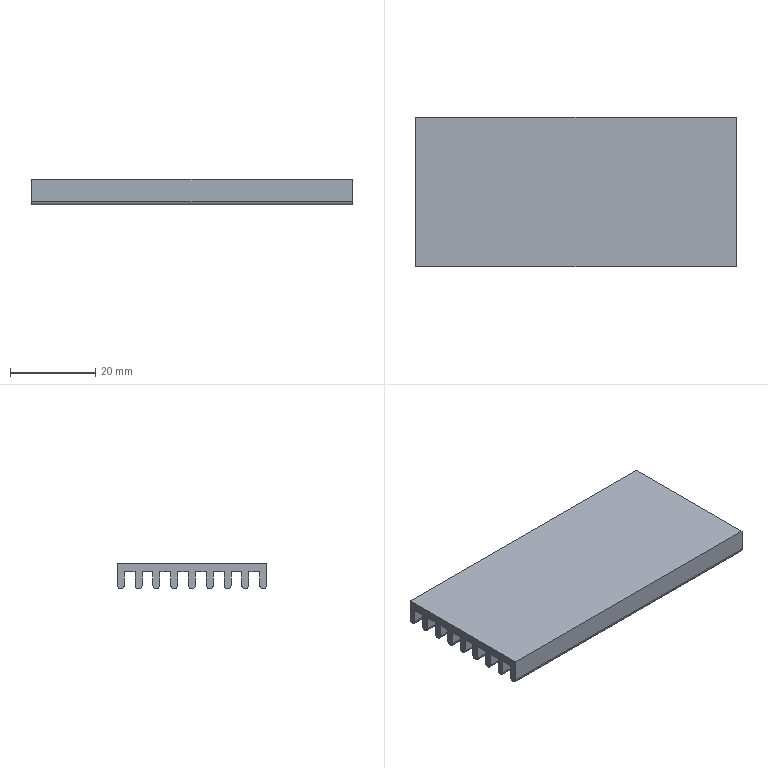Part | SolidWorks | features Fillet 9, Cut 1, Extrusion 1, LPattern 1 | 1 solid | 38 faces | box 75 x 35 x 6 mm | volume 9439 mm3 | plane 29 | cylinder 9 | commonest cylinder face diameters 1.62 x8 1.64 x1
STEP:
#1=CARTESIAN_POINT('',(37.5,-15.86,0.82));
#2=VERTEX_POINT('',#1);
#3=CARTESIAN_POINT('',(-37.5,-15.86,0.82));
#4=VERTEX_POINT('',#3);
#5=CARTESIAN_POINT('',(37.5,-15.86,0.82));
#6=DIRECTION('',(-1.,0.,0.));
#7=VECTOR('',#6,1000.);
#8=LINE('',#5,#7);
#9=EDGE_CURVE('',#2,#4,#8,.T.);
#10=ORIENTED_EDGE('',*,*,#9,.F.);
#11=CARTESIAN_POINT('',(37.5,-17.5,0.82));
#12=VERTEX_POINT('',#11);
#13=CARTESIAN_POINT('',(37.5,-16.68,0.82));
#14=DIRECTION('',(1.,0.,0.));
#15=DIRECTION('',(0.,-1.,0.));
#16=AXIS2_PLACEMENT_3D('',#13,#14,#15);
#17=CIRCLE('',#16,0.82);
#18=EDGE_CURVE('',#12,#2,#17,.T.);
#19=ORIENTED_EDGE('',*,*,#18,.F.);
#20=CARTESIAN_POINT('',(-37.5,-17.5,0.82));
#21=VERTEX_POINT('',#20);
#22=CARTESIAN_POINT('',(-37.5,-17.5,0.82));
#23=DIRECTION('',(1.,0.,0.));
#24=VECTOR('',#23,1000.);
#25=LINE('',#22,#24);
#26=EDGE_CURVE('',#21,#12,#25,.T.);
#27=ORIENTED_EDGE('',*,*,#26,.F.);
#28=CARTESIAN_POINT('',(-37.5,-16.68,0.82));
#29=DIRECTION('',(-1.,0.,0.));
#30=DIRECTION('',(0.,1.,0.));
#31=AXIS2_PLACEMENT_3D('',#28,#29,#30);
#32=CIRCLE('',#31,0.82);
#33=EDGE_CURVE('',#4,#21,#32,.T.);
#34=ORIENTED_EDGE('',*,*,#33,.F.);
#35=EDGE_LOOP('',(#10,#19,#27,#34));
#36=FACE_OUTER_BOUND('',#35,.T.);
#37=CARTESIAN_POINT('',(37.5,-16.68,0.82));
#38=DIRECTION('',(-1.,0.,0.));
#39=DIRECTION('',(0.,0.,1.));
#40=AXIS2_PLACEMENT_3D('',#37,#38,#39);
#41=CYLINDRICAL_SURFACE('',#40,0.82);
#42=ADVANCED_FACE('',(#36),#41,.T.);
#43=CARTESIAN_POINT('',(37.5,-11.69,0.81));
#44=VERTEX_POINT('',#43);
#45=CARTESIAN_POINT('',(-37.5,-11.69,0.81));
#46=VERTEX_POINT('',#45);
#47=CARTESIAN_POINT('',(37.5,-11.69,0.81));
#48=DIRECTION('',(-1.,0.,0.));
#49=VECTOR('',#48,1000.);
#50=LINE('',#47,#49);
#51=EDGE_CURVE('',#44,#46,#50,.T.);
#52=ORIENTED_EDGE('',*,*,#51,.F.);
#53=CARTESIAN_POINT('',(37.5,-13.31,0.81));
#54=VERTEX_POINT('',#53);
#55=CARTESIAN_POINT('',(37.5,-12.5,0.81));
#56=DIRECTION('',(1.,0.,0.));
#57=DIRECTION('',(0.,-1.,0.));
#58=AXIS2_PLACEMENT_3D('',#55,#56,#57);
#59=CIRCLE('',#58,0.81);
#60=EDGE_CURVE('',#54,#44,#59,.T.);
#61=ORIENTED_EDGE('',*,*,#60,.F.);
#62=CARTESIAN_POINT('',(-37.5,-13.31,0.81));
#63=VERTEX_POINT('',#62);
#64=CARTESIAN_POINT('',(37.5,-13.31,0.81));
#65=DIRECTION('',(1.,0.,0.));
#66=VECTOR('',#65,1000.);
#67=LINE('',#64,#66);
#68=EDGE_CURVE('',#63,#54,#67,.T.);
#69=ORIENTED_EDGE('',*,*,#68,.F.);
#70=CARTESIAN_POINT('',(-37.5,-12.5,0.81));
#71=DIRECTION('',(-1.,0.,0.));
#72=DIRECTION('',(0.,1.,0.));
#73=AXIS2_PLACEMENT_3D('',#70,#71,#72);
#74=CIRCLE('',#73,0.81);
#75=EDGE_CURVE('',#46,#63,#74,.T.);
#76=ORIENTED_EDGE('',*,*,#75,.F.);
#77=EDGE_LOOP('',(#52,#61,#69,#76));
#78=FACE_OUTER_BOUND('',#77,.T.);
#79=CARTESIAN_POINT('',(37.5,-12.5,0.81));
#80=DIRECTION('',(-1.,0.,0.));
#81=DIRECTION('',(0.,0.,1.));
#82=AXIS2_PLACEMENT_3D('',#79,#80,#81);
#83=CYLINDRICAL_SURFACE('',#82,0.81);
#84=ADVANCED_FACE('',(#78),#83,.T.);
#85=CARTESIAN_POINT('',(37.5,-7.52,0.81));
#86=VERTEX_POINT('',#85);
#87=CARTESIAN_POINT('',(-37.5,-7.52,0.81));
#88=VERTEX_POINT('',#87);
#89=CARTESIAN_POINT('',(37.5,-7.52,0.81));
#90=DIRECTION('',(-1.,0.,0.));
#91=VECTOR('',#90,1000.);
#92=LINE('',#89,#91);
#93=EDGE_CURVE('',#86,#88,#92,.T.);
#94=ORIENTED_EDGE('',*,*,#93,.F.);
#95=CARTESIAN_POINT('',(37.5,-9.14,0.81));
#96=VERTEX_POINT('',#95);
#97=CARTESIAN_POINT('',(37.5,-8.33,0.81));
#98=DIRECTION('',(1.,0.,0.));
#99=DIRECTION('',(0.,-1.,0.));
#100=AXIS2_PLACEMENT_3D('',#97,#98,#99);
#101=CIRCLE('',#100,0.81);
#102=EDGE_CURVE('',#96,#86,#101,.T.);
#103=ORIENTED_EDGE('',*,*,#102,.F.);
#104=CARTESIAN_POINT('',(-37.5,-9.14,0.81));
#105=VERTEX_POINT('',#104);
#106=CARTESIAN_POINT('',(37.5,-9.14,0.81));
#107=DIRECTION('',(1.,0.,0.));
#108=VECTOR('',#107,1000.);
#109=LINE('',#106,#108);
#110=EDGE_CURVE('',#105,#96,#109,.T.);
#111=ORIENTED_EDGE('',*,*,#110,.F.);
#112=CARTESIAN_POINT('',(-37.5,-8.33,0.81));
#113=DIRECTION('',(-1.,0.,0.));
#114=DIRECTION('',(0.,1.,0.));
#115=AXIS2_PLACEMENT_3D('',#112,#113,#114);
#116=CIRCLE('',#115,0.81);
#117=EDGE_CURVE('',#88,#105,#116,.T.);
#118=ORIENTED_EDGE('',*,*,#117,.F.);
#119=EDGE_LOOP('',(#94,#103,#111,#118));
#120=FACE_OUTER_BOUND('',#119,.T.);
#121=CARTESIAN_POINT('',(37.5,-8.33,0.81));
#122=DIRECTION('',(-1.,0.,0.));
#123=DIRECTION('',(0.,0.,1.));
#124=AXIS2_PLACEMENT_3D('',#121,#122,#123);
#125=CYLINDRICAL_SURFACE('',#124,0.81);
#126=ADVANCED_FACE('',(#120),#125,.T.);
#127=CARTESIAN_POINT('',(37.5,-3.35,0.81));
#128=VERTEX_POINT('',#127);
#129=CARTESIAN_POINT('',(-37.5,-3.35,0.81));
#130=VERTEX_POINT('',#129);
#131=CARTESIAN_POINT('',(37.5,-3.35,0.81));
#132=DIRECTION('',(-1.,0.,0.));
#133=VECTOR('',#132,1000.);
#134=LINE('',#131,#133);
#135=EDGE_CURVE('',#128,#130,#134,.T.);
#136=ORIENTED_EDGE('',*,*,#135,.F.);
#137=CARTESIAN_POINT('',(37.5,-4.97,0.81));
#138=VERTEX_POINT('',#137);
#139=CARTESIAN_POINT('',(37.5,-4.16,0.81));
#140=DIRECTION('',(1.,0.,0.));
#141=DIRECTION('',(0.,-1.,0.));
#142=AXIS2_PLACEMENT_3D('',#139,#140,#141);
#143=CIRCLE('',#142,0.81);
#144=EDGE_CURVE('',#138,#128,#143,.T.);
#145=ORIENTED_EDGE('',*,*,#144,.F.);
#146=CARTESIAN_POINT('',(-37.5,-4.97,0.81));
#147=VERTEX_POINT('',#146);
#148=CARTESIAN_POINT('',(37.5,-4.97,0.81));
#149=DIRECTION('',(1.,0.,0.));
#150=VECTOR('',#149,1000.);
#151=LINE('',#148,#150);
#152=EDGE_CURVE('',#147,#138,#151,.T.);
#153=ORIENTED_EDGE('',*,*,#152,.F.);
#154=CARTESIAN_POINT('',(-37.5,-4.16,0.81));
#155=DIRECTION('',(-1.,0.,0.));
#156=DIRECTION('',(0.,1.,0.));
#157=AXIS2_PLACEMENT_3D('',#154,#155,#156);
#158=CIRCLE('',#157,0.81);
#159=EDGE_CURVE('',#130,#147,#158,.T.);
#160=ORIENTED_EDGE('',*,*,#159,.F.);
#161=EDGE_LOOP('',(#136,#145,#153,#160));
#162=FACE_OUTER_BOUND('',#161,.T.);
#163=CARTESIAN_POINT('',(37.5,-4.16,0.81));
#164=DIRECTION('',(-1.,0.,0.));
#165=DIRECTION('',(0.,0.,1.));
#166=AXIS2_PLACEMENT_3D('',#163,#164,#165);
#167=CYLINDRICAL_SURFACE('',#166,0.81);
#168=ADVANCED_FACE('',(#162),#167,.T.);
#169=CARTESIAN_POINT('',(37.5,0.82,0.81));
#170=VERTEX_POINT('',#169);
#171=CARTESIAN_POINT('',(-37.5,0.82,0.81));
#172=VERTEX_POINT('',#171);
#173=CARTESIAN_POINT('',(37.5,0.82,0.81));
#174=DIRECTION('',(-1.,0.,0.));
#175=VECTOR('',#174,1000.);
#176=LINE('',#173,#175);
#177=EDGE_CURVE('',#170,#172,#176,.T.);
#178=ORIENTED_EDGE('',*,*,#177,.F.);
#179=CARTESIAN_POINT('',(37.5,-0.8,0.81));
#180=VERTEX_POINT('',#179);
#181=CARTESIAN_POINT('',(37.5,0.01,0.81));
#182=DIRECTION('',(1.,0.,0.));
#183=DIRECTION('',(0.,-1.,0.));
#184=AXIS2_PLACEMENT_3D('',#181,#182,#183);
#185=CIRCLE('',#184,0.81);
#186=EDGE_CURVE('',#180,#170,#185,.T.);
#187=ORIENTED_EDGE('',*,*,#186,.F.);
#188=CARTESIAN_POINT('',(-37.5,-0.8,0.81));
#189=VERTEX_POINT('',#188);
#190=CARTESIAN_POINT('',(37.5,-0.8,0.81));
#191=DIRECTION('',(1.,0.,0.));
#192=VECTOR('',#191,1000.);
#193=LINE('',#190,#192);
#194=EDGE_CURVE('',#189,#180,#193,.T.);
#195=ORIENTED_EDGE('',*,*,#194,.F.);
#196=CARTESIAN_POINT('',(-37.5,0.01,0.81));
#197=DIRECTION('',(-1.,0.,0.));
#198=DIRECTION('',(0.,1.,0.));
#199=AXIS2_PLACEMENT_3D('',#196,#197,#198);
#200=CIRCLE('',#199,0.81);
#201=EDGE_CURVE('',#172,#189,#200,.T.);
#202=ORIENTED_EDGE('',*,*,#201,.F.);
#203=EDGE_LOOP('',(#178,#187,#195,#202));
#204=FACE_OUTER_BOUND('',#203,.T.);
#205=CARTESIAN_POINT('',(37.5,0.01,0.81));
#206=DIRECTION('',(-1.,0.,0.));
#207=DIRECTION('',(0.,0.,1.));
#208=AXIS2_PLACEMENT_3D('',#205,#206,#207);
#209=CYLINDRICAL_SURFACE('',#208,0.81);
#210=ADVANCED_FACE('',(#204),#209,.T.);
#211=CARTESIAN_POINT('',(37.5,4.99,0.81));
#212=VERTEX_POINT('',#211);
#213=CARTESIAN_POINT('',(-37.5,4.99,0.81));
#214=VERTEX_POINT('',#213);
#215=CARTESIAN_POINT('',(37.5,4.99,0.81));
#216=DIRECTION('',(-1.,0.,0.));
#217=VECTOR('',#216,1000.);
#218=LINE('',#215,#217);
#219=EDGE_CURVE('',#212,#214,#218,.T.);
#220=ORIENTED_EDGE('',*,*,#219,.F.);
#221=CARTESIAN_POINT('',(37.5,3.37,0.81));
#222=VERTEX_POINT('',#221);
#223=CARTESIAN_POINT('',(37.5,4.18,0.81));
#224=DIRECTION('',(1.,0.,0.));
#225=DIRECTION('',(0.,-1.,0.));
#226=AXIS2_PLACEMENT_3D('',#223,#224,#225);
#227=CIRCLE('',#226,0.81);
#228=EDGE_CURVE('',#222,#212,#227,.T.);
#229=ORIENTED_EDGE('',*,*,#228,.F.);
#230=CARTESIAN_POINT('',(-37.5,3.37,0.81));
#231=VERTEX_POINT('',#230);
#232=CARTESIAN_POINT('',(37.5,3.37,0.81));
#233=DIRECTION('',(1.,0.,0.));
#234=VECTOR('',#233,1000.);
#235=LINE('',#232,#234);
#236=EDGE_CURVE('',#231,#222,#235,.T.);
#237=ORIENTED_EDGE('',*,*,#236,.F.);
#238=CARTESIAN_POINT('',(-37.5,4.18,0.81));
#239=DIRECTION('',(-1.,0.,0.));
#240=DIRECTION('',(0.,1.,0.));
#241=AXIS2_PLACEMENT_3D('',#238,#239,#240);
#242=CIRCLE('',#241,0.81);
#243=EDGE_CURVE('',#214,#231,#242,.T.);
#244=ORIENTED_EDGE('',*,*,#243,.F.);
#245=EDGE_LOOP('',(#220,#229,#237,#244));
#246=FACE_OUTER_BOUND('',#245,.T.);
#247=CARTESIAN_POINT('',(37.5,4.18,0.81));
#248=DIRECTION('',(-1.,0.,0.));
#249=DIRECTION('',(0.,0.,1.));
#250=AXIS2_PLACEMENT_3D('',#247,#248,#249);
#251=CYLINDRICAL_SURFACE('',#250,0.81);
#252=ADVANCED_FACE('',(#246),#251,.T.);
#253=CARTESIAN_POINT('',(37.5,9.16,0.81));
#254=VERTEX_POINT('',#253);
#255=CARTESIAN_POINT('',(-37.5,9.16,0.81));
#256=VERTEX_POINT('',#255);
#257=CARTESIAN_POINT('',(37.5,9.16,0.81));
#258=DIRECTION('',(-1.,0.,0.));
#259=VECTOR('',#258,1000.);
#260=LINE('',#257,#259);
#261=EDGE_CURVE('',#254,#256,#260,.T.);
#262=ORIENTED_EDGE('',*,*,#261,.F.);
#263=CARTESIAN_POINT('',(37.5,7.54,0.81));
#264=VERTEX_POINT('',#263);
#265=CARTESIAN_POINT('',(37.5,8.35,0.81));
#266=DIRECTION('',(1.,0.,0.));
#267=DIRECTION('',(0.,-1.,0.));
#268=AXIS2_PLACEMENT_3D('',#265,#266,#267);
#269=CIRCLE('',#268,0.81);
#270=EDGE_CURVE('',#264,#254,#269,.T.);
#271=ORIENTED_EDGE('',*,*,#270,.F.);
#272=CARTESIAN_POINT('',(-37.5,7.54,0.81));
#273=VERTEX_POINT('',#272);
#274=CARTESIAN_POINT('',(37.5,7.54,0.81));
#275=DIRECTION('',(1.,0.,0.));
#276=VECTOR('',#275,1000.);
#277=LINE('',#274,#276);
#278=EDGE_CURVE('',#273,#264,#277,.T.);
#279=ORIENTED_EDGE('',*,*,#278,.F.);
#280=CARTESIAN_POINT('',(-37.5,8.35,0.81));
#281=DIRECTION('',(-1.,0.,0.));
#282=DIRECTION('',(0.,1.,0.));
#283=AXIS2_PLACEMENT_3D('',#280,#281,#282);
#284=CIRCLE('',#283,0.81);
#285=EDGE_CURVE('',#256,#273,#284,.T.);
#286=ORIENTED_EDGE('',*,*,#285,.F.);
#287=EDGE_LOOP('',(#262,#271,#279,#286));
#288=FACE_OUTER_BOUND('',#287,.T.);
#289=CARTESIAN_POINT('',(37.5,8.35,0.81));
#290=DIRECTION('',(-1.,0.,0.));
#291=DIRECTION('',(0.,0.,1.));
#292=AXIS2_PLACEMENT_3D('',#289,#290,#291);
#293=CYLINDRICAL_SURFACE('',#292,0.81);
#294=ADVANCED_FACE('',(#288),#293,.T.);
#295=CARTESIAN_POINT('',(37.5,13.33,0.81));
#296=VERTEX_POINT('',#295);
#297=CARTESIAN_POINT('',(-37.5,13.33,0.81));
#298=VERTEX_POINT('',#297);
#299=CARTESIAN_POINT('',(37.5,13.33,0.81));
#300=DIRECTION('',(-1.,0.,0.));
#301=VECTOR('',#300,1000.);
#302=LINE('',#299,#301);
#303=EDGE_CURVE('',#296,#298,#302,.T.);
#304=ORIENTED_EDGE('',*,*,#303,.F.);
#305=CARTESIAN_POINT('',(37.5,11.71,0.81));
#306=VERTEX_POINT('',#305);
#307=CARTESIAN_POINT('',(37.5,12.52,0.81));
#308=DIRECTION('',(1.,0.,0.));
#309=DIRECTION('',(0.,-1.,0.));
#310=AXIS2_PLACEMENT_3D('',#307,#308,#309);
#311=CIRCLE('',#310,0.81);
#312=EDGE_CURVE('',#306,#296,#311,.T.);
#313=ORIENTED_EDGE('',*,*,#312,.F.);
#314=CARTESIAN_POINT('',(-37.5,11.71,0.81));
#315=VERTEX_POINT('',#314);
#316=CARTESIAN_POINT('',(37.5,11.71,0.81));
#317=DIRECTION('',(1.,0.,0.));
#318=VECTOR('',#317,1000.);
#319=LINE('',#316,#318);
#320=EDGE_CURVE('',#315,#306,#319,.T.);
#321=ORIENTED_EDGE('',*,*,#320,.F.);
#322=CARTESIAN_POINT('',(-37.5,12.52,0.81));
#323=DIRECTION('',(-1.,0.,0.));
#324=DIRECTION('',(0.,1.,0.));
#325=AXIS2_PLACEMENT_3D('',#322,#323,#324);
#326=CIRCLE('',#325,0.81);
#327=EDGE_CURVE('',#298,#315,#326,.T.);
#328=ORIENTED_EDGE('',*,*,#327,.F.);
#329=EDGE_LOOP('',(#304,#313,#321,#328));
#330=FACE_OUTER_BOUND('',#329,.T.);
#331=CARTESIAN_POINT('',(37.5,12.52,0.81));
#332=DIRECTION('',(-1.,0.,0.));
#333=DIRECTION('',(0.,0.,1.));
#334=AXIS2_PLACEMENT_3D('',#331,#332,#333);
#335=CYLINDRICAL_SURFACE('',#334,0.81);
#336=ADVANCED_FACE('',(#330),#335,.T.);
#337=CARTESIAN_POINT('',(37.5,17.5,0.81));
#338=VERTEX_POINT('',#337);
#339=CARTESIAN_POINT('',(-37.5,17.5,0.81));
#340=VERTEX_POINT('',#339);
#341=CARTESIAN_POINT('',(-37.5,17.5,0.81));
#342=DIRECTION('',(-1.,0.,0.));
#343=VECTOR('',#342,1000.);
#344=LINE('',#341,#343);
#345=EDGE_CURVE('',#338,#340,#344,.T.);
#346=ORIENTED_EDGE('',*,*,#345,.F.);
#347=CARTESIAN_POINT('',(37.5,15.88,0.81));
#348=VERTEX_POINT('',#347);
#349=CARTESIAN_POINT('',(37.5,16.69,0.81));
#350=DIRECTION('',(1.,0.,0.));
#351=DIRECTION('',(0.,-1.,0.));
#352=AXIS2_PLACEMENT_3D('',#349,#350,#351);
#353=CIRCLE('',#352,0.81);
#354=EDGE_CURVE('',#348,#338,#353,.T.);
#355=ORIENTED_EDGE('',*,*,#354,.F.);
#356=CARTESIAN_POINT('',(-37.5,15.88,0.81));
#357=VERTEX_POINT('',#356);
#358=CARTESIAN_POINT('',(37.5,15.88,0.81));
#359=DIRECTION('',(1.,0.,0.));
#360=VECTOR('',#359,1000.);
#361=LINE('',#358,#360);
#362=EDGE_CURVE('',#357,#348,#361,.T.);
#363=ORIENTED_EDGE('',*,*,#362,.F.);
#364=CARTESIAN_POINT('',(-37.5,16.69,0.81));
#365=DIRECTION('',(-1.,0.,0.));
#366=DIRECTION('',(0.,1.,0.));
#367=AXIS2_PLACEMENT_3D('',#364,#365,#366);
#368=CIRCLE('',#367,0.81);
#369=EDGE_CURVE('',#340,#357,#368,.T.);
#370=ORIENTED_EDGE('',*,*,#369,.F.);
#371=EDGE_LOOP('',(#346,#355,#363,#370));
#372=FACE_OUTER_BOUND('',#371,.T.);
#373=CARTESIAN_POINT('',(37.5,16.69,0.81));
#374=DIRECTION('',(-1.,0.,0.));
#375=DIRECTION('',(0.,-1.,0.));
#376=AXIS2_PLACEMENT_3D('',#373,#374,#375);
#377=CYLINDRICAL_SURFACE('',#376,0.81);
#378=ADVANCED_FACE('',(#372),#377,.T.);
#379=CARTESIAN_POINT('',(-37.5,-15.86,4.));
#380=VERTEX_POINT('',#379);
#381=CARTESIAN_POINT('',(-37.5,-15.86,4.));
#382=DIRECTION('',(0.,0.,-1.));
#383=VECTOR('',#382,1000.);
#384=LINE('',#381,#383);
#385=EDGE_CURVE('',#380,#4,#384,.T.);
#386=ORIENTED_EDGE('',*,*,#385,.T.);
#387=ORIENTED_EDGE('',*,*,#33,.T.);
#388=CARTESIAN_POINT('',(-37.5,-17.5,6.));
#389=VERTEX_POINT('',#388);
#390=CARTESIAN_POINT('',(-37.5,-17.5,6.));
#391=DIRECTION('',(0.,0.,-1.));
#392=VECTOR('',#391,1000.);
#393=LINE('',#390,#392);
#394=EDGE_CURVE('',#389,#21,#393,.T.);
#395=ORIENTED_EDGE('',*,*,#394,.F.);
#396=CARTESIAN_POINT('',(-37.5,17.5,6.));
#397=VERTEX_POINT('',#396);
#398=CARTESIAN_POINT('',(-37.5,17.5,6.));
#399=DIRECTION('',(0.,-1.,0.));
#400=VECTOR('',#399,1000.);
#401=LINE('',#398,#400);
#402=EDGE_CURVE('',#397,#389,#401,.T.);
#403=ORIENTED_EDGE('',*,*,#402,.F.);
#404=CARTESIAN_POINT('',(-37.5,17.5,6.));
#405=DIRECTION('',(0.,0.,-1.));
#406=VECTOR('',#405,1000.);
#407=LINE('',#404,#406);
#408=EDGE_CURVE('',#397,#340,#407,.T.);
#409=ORIENTED_EDGE('',*,*,#408,.T.);
#410=ORIENTED_EDGE('',*,*,#369,.T.);
#411=CARTESIAN_POINT('',(-37.5,15.88,4.));
#412=VERTEX_POINT('',#411);
#413=CARTESIAN_POINT('',(-37.5,15.88,4.));
#414=DIRECTION('',(0.,0.,-1.));
#415=VECTOR('',#414,1000.);
#416=LINE('',#413,#415);
#417=EDGE_CURVE('',#412,#357,#416,.T.);
#418=ORIENTED_EDGE('',*,*,#417,.F.);
#419=CARTESIAN_POINT('',(-37.5,13.33,4.));
#420=VERTEX_POINT('',#419);
#421=CARTESIAN_POINT('',(-37.5,15.88,4.));
#422=DIRECTION('',(0.,1.,0.));
#423=VECTOR('',#422,1000.);
#424=LINE('',#421,#423);
#425=EDGE_CURVE('',#420,#412,#424,.T.);
#426=ORIENTED_EDGE('',*,*,#425,.F.);
#427=CARTESIAN_POINT('',(-37.5,13.33,4.));
#428=DIRECTION('',(0.,0.,-1.));
#429=VECTOR('',#428,1000.);
#430=LINE('',#427,#429);
#431=EDGE_CURVE('',#420,#298,#430,.T.);
#432=ORIENTED_EDGE('',*,*,#431,.T.);
#433=ORIENTED_EDGE('',*,*,#327,.T.);
#434=CARTESIAN_POINT('',(-37.5,11.71,4.));
#435=VERTEX_POINT('',#434);
#436=CARTESIAN_POINT('',(-37.5,11.71,4.));
#437=DIRECTION('',(0.,0.,-1.));
#438=VECTOR('',#437,1000.);
#439=LINE('',#436,#438);
#440=EDGE_CURVE('',#435,#315,#439,.T.);
#441=ORIENTED_EDGE('',*,*,#440,.F.);
#442=CARTESIAN_POINT('',(-37.5,9.16,4.));
#443=VERTEX_POINT('',#442);
#444=CARTESIAN_POINT('',(-37.5,11.71,4.));
#445=DIRECTION('',(0.,1.,0.));
#446=VECTOR('',#445,1000.);
#447=LINE('',#444,#446);
#448=EDGE_CURVE('',#443,#435,#447,.T.);
#449=ORIENTED_EDGE('',*,*,#448,.F.);
#450=CARTESIAN_POINT('',(-37.5,9.16,4.));
#451=DIRECTION('',(0.,0.,-1.));
#452=VECTOR('',#451,1000.);
#453=LINE('',#450,#452);
#454=EDGE_CURVE('',#443,#256,#453,.T.);
#455=ORIENTED_EDGE('',*,*,#454,.T.);
#456=ORIENTED_EDGE('',*,*,#285,.T.);
#457=CARTESIAN_POINT('',(-37.5,7.54,4.));
#458=VERTEX_POINT('',#457);
#459=CARTESIAN_POINT('',(-37.5,7.54,4.));
#460=DIRECTION('',(0.,0.,-1.));
#461=VECTOR('',#460,1000.);
#462=LINE('',#459,#461);
#463=EDGE_CURVE('',#458,#273,#462,.T.);
#464=ORIENTED_EDGE('',*,*,#463,.F.);
#465=CARTESIAN_POINT('',(-37.5,4.99,4.));
#466=VERTEX_POINT('',#465);
#467=CARTESIAN_POINT('',(-37.5,7.54,4.));
#468=DIRECTION('',(0.,1.,0.));
#469=VECTOR('',#468,1000.);
#470=LINE('',#467,#469);
#471=EDGE_CURVE('',#466,#458,#470,.T.);
#472=ORIENTED_EDGE('',*,*,#471,.F.);
#473=CARTESIAN_POINT('',(-37.5,4.99,4.));
#474=DIRECTION('',(0.,0.,-1.));
#475=VECTOR('',#474,1000.);
#476=LINE('',#473,#475);
#477=EDGE_CURVE('',#466,#214,#476,.T.);
#478=ORIENTED_EDGE('',*,*,#477,.T.);
#479=ORIENTED_EDGE('',*,*,#243,.T.);
#480=CARTESIAN_POINT('',(-37.5,3.37,4.));
#481=VERTEX_POINT('',#480);
#482=CARTESIAN_POINT('',(-37.5,3.37,4.));
#483=DIRECTION('',(0.,0.,-1.));
#484=VECTOR('',#483,1000.);
#485=LINE('',#482,#484);
#486=EDGE_CURVE('',#481,#231,#485,.T.);
#487=ORIENTED_EDGE('',*,*,#486,.F.);
#488=CARTESIAN_POINT('',(-37.5,0.82,4.));
#489=VERTEX_POINT('',#488);
#490=CARTESIAN_POINT('',(-37.5,3.37,4.));
#491=DIRECTION('',(0.,1.,0.));
#492=VECTOR('',#491,1000.);
#493=LINE('',#490,#492);
#494=EDGE_CURVE('',#489,#481,#493,.T.);
#495=ORIENTED_EDGE('',*,*,#494,.F.);
#496=CARTESIAN_POINT('',(-37.5,0.82,4.));
#497=DIRECTION('',(0.,0.,-1.));
#498=VECTOR('',#497,1000.);
#499=LINE('',#496,#498);
#500=EDGE_CURVE('',#489,#172,#499,.T.);
#501=ORIENTED_EDGE('',*,*,#500,.T.);
#502=ORIENTED_EDGE('',*,*,#201,.T.);
#503=CARTESIAN_POINT('',(-37.5,-0.8,4.));
#504=VERTEX_POINT('',#503);
#505=CARTESIAN_POINT('',(-37.5,-0.8,4.));
#506=DIRECTION('',(0.,0.,-1.));
#507=VECTOR('',#506,1000.);
#508=LINE('',#505,#507);
#509=EDGE_CURVE('',#504,#189,#508,.T.);
#510=ORIENTED_EDGE('',*,*,#509,.F.);
#511=CARTESIAN_POINT('',(-37.5,-3.35,4.));
#512=VERTEX_POINT('',#511);
#513=CARTESIAN_POINT('',(-37.5,-0.8,4.));
#514=DIRECTION('',(0.,1.,0.));
#515=VECTOR('',#514,1000.);
#516=LINE('',#513,#515);
#517=EDGE_CURVE('',#512,#504,#516,.T.);
#518=ORIENTED_EDGE('',*,*,#517,.F.);
#519=CARTESIAN_POINT('',(-37.5,-3.35,4.));
#520=DIRECTION('',(0.,0.,-1.));
#521=VECTOR('',#520,1000.);
#522=LINE('',#519,#521);
#523=EDGE_CURVE('',#512,#130,#522,.T.);
#524=ORIENTED_EDGE('',*,*,#523,.T.);
#525=ORIENTED_EDGE('',*,*,#159,.T.);
#526=CARTESIAN_POINT('',(-37.5,-4.97,4.));
#527=VERTEX_POINT('',#526);
#528=CARTESIAN_POINT('',(-37.5,-4.97,4.));
#529=DIRECTION('',(0.,0.,-1.));
#530=VECTOR('',#529,1000.);
#531=LINE('',#528,#530);
#532=EDGE_CURVE('',#527,#147,#531,.T.);
#533=ORIENTED_EDGE('',*,*,#532,.F.);
#534=CARTESIAN_POINT('',(-37.5,-7.52,4.));
#535=VERTEX_POINT('',#534);
#536=CARTESIAN_POINT('',(-37.5,-4.97,4.));
#537=DIRECTION('',(0.,1.,0.));
#538=VECTOR('',#537,1000.);
#539=LINE('',#536,#538);
#540=EDGE_CURVE('',#535,#527,#539,.T.);
#541=ORIENTED_EDGE('',*,*,#540,.F.);
#542=CARTESIAN_POINT('',(-37.5,-7.52,4.));
#543=DIRECTION('',(0.,0.,-1.));
#544=VECTOR('',#543,1000.);
#545=LINE('',#542,#544);
#546=EDGE_CURVE('',#535,#88,#545,.T.);
#547=ORIENTED_EDGE('',*,*,#546,.T.);
#548=ORIENTED_EDGE('',*,*,#117,.T.);
#549=CARTESIAN_POINT('',(-37.5,-9.14,4.));
#550=VERTEX_POINT('',#549);
#551=CARTESIAN_POINT('',(-37.5,-9.14,4.));
#552=DIRECTION('',(0.,0.,-1.));
#553=VECTOR('',#552,1000.);
#554=LINE('',#551,#553);
#555=EDGE_CURVE('',#550,#105,#554,.T.);
#556=ORIENTED_EDGE('',*,*,#555,.F.);
#557=CARTESIAN_POINT('',(-37.5,-11.69,4.));
#558=VERTEX_POINT('',#557);
#559=CARTESIAN_POINT('',(-37.5,-9.14,4.));
#560=DIRECTION('',(0.,1.,0.));
#561=VECTOR('',#560,1000.);
#562=LINE('',#559,#561);
#563=EDGE_CURVE('',#558,#550,#562,.T.);
#564=ORIENTED_EDGE('',*,*,#563,.F.);
#565=CARTESIAN_POINT('',(-37.5,-11.69,4.));
#566=DIRECTION('',(0.,0.,-1.));
#567=VECTOR('',#566,1000.);
#568=LINE('',#565,#567);
#569=EDGE_CURVE('',#558,#46,#568,.T.);
#570=ORIENTED_EDGE('',*,*,#569,.T.);
#571=ORIENTED_EDGE('',*,*,#75,.T.);
#572=CARTESIAN_POINT('',(-37.5,-13.31,4.));
#573=VERTEX_POINT('',#572);
#574=CARTESIAN_POINT('',(-37.5,-13.31,4.));
#575=DIRECTION('',(0.,0.,-1.));
#576=VECTOR('',#575,1000.);
#577=LINE('',#574,#576);
#578=EDGE_CURVE('',#573,#63,#577,.T.);
#579=ORIENTED_EDGE('',*,*,#578,.F.);
#580=CARTESIAN_POINT('',(-37.5,-13.31,4.));
#581=DIRECTION('',(0.,1.,0.));
#582=VECTOR('',#581,1000.);
#583=LINE('',#580,#582);
#584=EDGE_CURVE('',#380,#573,#583,.T.);
#585=ORIENTED_EDGE('',*,*,#584,.F.);
#586=EDGE_LOOP('',(#386,#387,#395,#403,#409,#410,#418,#426,#432,#433,#441,#449,#455,#456,#464,#472,#478,#479,#487,#495,#501,#502,#510,#518,#524,#525,#533,#541,#547,#548,#556,#564,#570,#571,#579,#585));
#587=FACE_OUTER_BOUND('',#586,.T.);
#588=CARTESIAN_POINT('',(-37.5,17.5,6.));
#589=DIRECTION('',(1.,0.,0.));
#590=DIRECTION('',(0.,1.,0.));
#591=AXIS2_PLACEMENT_3D('',#588,#589,#590);
#592=PLANE('',#591);
#593=ADVANCED_FACE('',(#587),#592,.F.);
#594=ORIENTED_EDGE('',*,*,#394,.T.);
#595=ORIENTED_EDGE('',*,*,#26,.T.);
#596=CARTESIAN_POINT('',(37.5,-17.5,6.));
#597=VERTEX_POINT('',#596);
#598=CARTESIAN_POINT('',(37.5,-17.5,6.));
#599=DIRECTION('',(0.,0.,-1.));
#600=VECTOR('',#599,1000.);
#601=LINE('',#598,#600);
#602=EDGE_CURVE('',#597,#12,#601,.T.);
#603=ORIENTED_EDGE('',*,*,#602,.F.);
#604=CARTESIAN_POINT('',(-37.5,-17.5,6.));
#605=DIRECTION('',(1.,0.,0.));
#606=VECTOR('',#605,1000.);
#607=LINE('',#604,#606);
#608=EDGE_CURVE('',#389,#597,#607,.T.);
#609=ORIENTED_EDGE('',*,*,#608,.F.);
#610=EDGE_LOOP('',(#594,#595,#603,#609));
#611=FACE_OUTER_BOUND('',#610,.T.);
#612=CARTESIAN_POINT('',(-37.5,-17.5,6.));
#613=DIRECTION('',(0.,1.,0.));
#614=DIRECTION('',(0.,0.,1.));
#615=AXIS2_PLACEMENT_3D('',#612,#613,#614);
#616=PLANE('',#615);
#617=ADVANCED_FACE('',(#611),#616,.F.);
#618=ORIENTED_EDGE('',*,*,#602,.T.);
#619=ORIENTED_EDGE('',*,*,#18,.T.);
#620=CARTESIAN_POINT('',(37.5,-15.86,4.));
#621=VERTEX_POINT('',#620);
#622=CARTESIAN_POINT('',(37.5,-15.86,4.));
#623=DIRECTION('',(0.,0.,-1.));
#624=VECTOR('',#623,1000.);
#625=LINE('',#622,#624);
#626=EDGE_CURVE('',#621,#2,#625,.T.);
#627=ORIENTED_EDGE('',*,*,#626,.F.);
#628=CARTESIAN_POINT('',(37.5,-13.31,4.));
#629=VERTEX_POINT('',#628);
#630=CARTESIAN_POINT('',(37.5,-15.86,4.));
#631=DIRECTION('',(0.,-1.,0.));
#632=VECTOR('',#631,1000.);
#633=LINE('',#630,#632);
#634=EDGE_CURVE('',#629,#621,#633,.T.);
#635=ORIENTED_EDGE('',*,*,#634,.F.);
#636=CARTESIAN_POINT('',(37.5,-13.31,4.));
#637=DIRECTION('',(0.,0.,-1.));
#638=VECTOR('',#637,1000.);
#639=LINE('',#636,#638);
#640=EDGE_CURVE('',#629,#54,#639,.T.);
#641=ORIENTED_EDGE('',*,*,#640,.T.);
#642=ORIENTED_EDGE('',*,*,#60,.T.);
#643=CARTESIAN_POINT('',(37.5,-11.69,4.));
#644=VERTEX_POINT('',#643);
#645=CARTESIAN_POINT('',(37.5,-11.69,4.));
#646=DIRECTION('',(0.,0.,-1.));
#647=VECTOR('',#646,1000.);
#648=LINE('',#645,#647);
#649=EDGE_CURVE('',#644,#44,#648,.T.);
#650=ORIENTED_EDGE('',*,*,#649,.F.);
#651=CARTESIAN_POINT('',(37.5,-9.14,4.));
#652=VERTEX_POINT('',#651);
#653=CARTESIAN_POINT('',(37.5,-11.69,4.));
#654=DIRECTION('',(0.,-1.,0.));
#655=VECTOR('',#654,1000.);
#656=LINE('',#653,#655);
#657=EDGE_CURVE('',#652,#644,#656,.T.);
#658=ORIENTED_EDGE('',*,*,#657,.F.);
#659=CARTESIAN_POINT('',(37.5,-9.14,4.));
#660=DIRECTION('',(0.,0.,-1.));
#661=VECTOR('',#660,1000.);
#662=LINE('',#659,#661);
#663=EDGE_CURVE('',#652,#96,#662,.T.);
#664=ORIENTED_EDGE('',*,*,#663,.T.);
#665=ORIENTED_EDGE('',*,*,#102,.T.);
#666=CARTESIAN_POINT('',(37.5,-7.52,4.));
#667=VERTEX_POINT('',#666);
#668=CARTESIAN_POINT('',(37.5,-7.52,4.));
#669=DIRECTION('',(0.,0.,-1.));
#670=VECTOR('',#669,1000.);
#671=LINE('',#668,#670);
#672=EDGE_CURVE('',#667,#86,#671,.T.);
#673=ORIENTED_EDGE('',*,*,#672,.F.);
#674=CARTESIAN_POINT('',(37.5,-4.97,4.));
#675=VERTEX_POINT('',#674);
#676=CARTESIAN_POINT('',(37.5,-7.52,4.));
#677=DIRECTION('',(0.,-1.,0.));
#678=VECTOR('',#677,1000.);
#679=LINE('',#676,#678);
#680=EDGE_CURVE('',#675,#667,#679,.T.);
#681=ORIENTED_EDGE('',*,*,#680,.F.);
#682=CARTESIAN_POINT('',(37.5,-4.97,4.));
#683=DIRECTION('',(0.,0.,-1.));
#684=VECTOR('',#683,1000.);
#685=LINE('',#682,#684);
#686=EDGE_CURVE('',#675,#138,#685,.T.);
#687=ORIENTED_EDGE('',*,*,#686,.T.);
#688=ORIENTED_EDGE('',*,*,#144,.T.);
#689=CARTESIAN_POINT('',(37.5,-3.35,4.));
#690=VERTEX_POINT('',#689);
#691=CARTESIAN_POINT('',(37.5,-3.35,4.));
#692=DIRECTION('',(0.,0.,-1.));
#693=VECTOR('',#692,1000.);
#694=LINE('',#691,#693);
#695=EDGE_CURVE('',#690,#128,#694,.T.);
#696=ORIENTED_EDGE('',*,*,#695,.F.);
#697=CARTESIAN_POINT('',(37.5,-0.8,4.));
#698=VERTEX_POINT('',#697);
#699=CARTESIAN_POINT('',(37.5,-3.35,4.));
#700=DIRECTION('',(0.,-1.,0.));
#701=VECTOR('',#700,1000.);
#702=LINE('',#699,#701);
#703=EDGE_CURVE('',#698,#690,#702,.T.);
#704=ORIENTED_EDGE('',*,*,#703,.F.);
#705=CARTESIAN_POINT('',(37.5,-0.8,4.));
#706=DIRECTION('',(0.,0.,-1.));
#707=VECTOR('',#706,1000.);
#708=LINE('',#705,#707);
#709=EDGE_CURVE('',#698,#180,#708,.T.);
#710=ORIENTED_EDGE('',*,*,#709,.T.);
#711=ORIENTED_EDGE('',*,*,#186,.T.);
#712=CARTESIAN_POINT('',(37.5,0.82,4.));
#713=VERTEX_POINT('',#712);
#714=CARTESIAN_POINT('',(37.5,0.82,4.));
#715=DIRECTION('',(0.,0.,-1.));
#716=VECTOR('',#715,1000.);
#717=LINE('',#714,#716);
#718=EDGE_CURVE('',#713,#170,#717,.T.);
#719=ORIENTED_EDGE('',*,*,#718,.F.);
#720=CARTESIAN_POINT('',(37.5,3.37,4.));
#721=VERTEX_POINT('',#720);
#722=CARTESIAN_POINT('',(37.5,0.82,4.));
#723=DIRECTION('',(0.,-1.,0.));
#724=VECTOR('',#723,1000.);
#725=LINE('',#722,#724);
#726=EDGE_CURVE('',#721,#713,#725,.T.);
#727=ORIENTED_EDGE('',*,*,#726,.F.);
#728=CARTESIAN_POINT('',(37.5,3.37,4.));
#729=DIRECTION('',(0.,0.,-1.));
#730=VECTOR('',#729,1000.);
#731=LINE('',#728,#730);
#732=EDGE_CURVE('',#721,#222,#731,.T.);
#733=ORIENTED_EDGE('',*,*,#732,.T.);
#734=ORIENTED_EDGE('',*,*,#228,.T.);
#735=CARTESIAN_POINT('',(37.5,4.99,4.));
#736=VERTEX_POINT('',#735);
#737=CARTESIAN_POINT('',(37.5,4.99,4.));
#738=DIRECTION('',(0.,0.,-1.));
#739=VECTOR('',#738,1000.);
#740=LINE('',#737,#739);
#741=EDGE_CURVE('',#736,#212,#740,.T.);
#742=ORIENTED_EDGE('',*,*,#741,.F.);
#743=CARTESIAN_POINT('',(37.5,7.54,4.));
#744=VERTEX_POINT('',#743);
#745=CARTESIAN_POINT('',(37.5,4.99,4.));
#746=DIRECTION('',(0.,-1.,0.));
#747=VECTOR('',#746,1000.);
#748=LINE('',#745,#747);
#749=EDGE_CURVE('',#744,#736,#748,.T.);
#750=ORIENTED_EDGE('',*,*,#749,.F.);
#751=CARTESIAN_POINT('',(37.5,7.54,4.));
#752=DIRECTION('',(0.,0.,-1.));
#753=VECTOR('',#752,1000.);
#754=LINE('',#751,#753);
#755=EDGE_CURVE('',#744,#264,#754,.T.);
#756=ORIENTED_EDGE('',*,*,#755,.T.);
#757=ORIENTED_EDGE('',*,*,#270,.T.);
#758=CARTESIAN_POINT('',(37.5,9.16,4.));
#759=VERTEX_POINT('',#758);
#760=CARTESIAN_POINT('',(37.5,9.16,4.));
#761=DIRECTION('',(0.,0.,-1.));
#762=VECTOR('',#761,1000.);
#763=LINE('',#760,#762);
#764=EDGE_CURVE('',#759,#254,#763,.T.);
#765=ORIENTED_EDGE('',*,*,#764,.F.);
#766=CARTESIAN_POINT('',(37.5,11.71,4.));
#767=VERTEX_POINT('',#766);
#768=CARTESIAN_POINT('',(37.5,9.16,4.));
#769=DIRECTION('',(0.,-1.,0.));
#770=VECTOR('',#769,1000.);
#771=LINE('',#768,#770);
#772=EDGE_CURVE('',#767,#759,#771,.T.);
#773=ORIENTED_EDGE('',*,*,#772,.F.);
#774=CARTESIAN_POINT('',(37.5,11.71,4.));
#775=DIRECTION('',(0.,0.,-1.));
#776=VECTOR('',#775,1000.);
#777=LINE('',#774,#776);
#778=EDGE_CURVE('',#767,#306,#777,.T.);
#779=ORIENTED_EDGE('',*,*,#778,.T.);
#780=ORIENTED_EDGE('',*,*,#312,.T.);
#781=CARTESIAN_POINT('',(37.5,13.33,4.));
#782=VERTEX_POINT('',#781);
#783=CARTESIAN_POINT('',(37.5,13.33,4.));
#784=DIRECTION('',(0.,0.,-1.));
#785=VECTOR('',#784,1000.);
#786=LINE('',#783,#785);
#787=EDGE_CURVE('',#782,#296,#786,.T.);
#788=ORIENTED_EDGE('',*,*,#787,.F.);
#789=CARTESIAN_POINT('',(37.5,15.88,4.));
#790=VERTEX_POINT('',#789);
#791=CARTESIAN_POINT('',(37.5,13.33,4.));
#792=DIRECTION('',(0.,-1.,0.));
#793=VECTOR('',#792,1000.);
#794=LINE('',#791,#793);
#795=EDGE_CURVE('',#790,#782,#794,.T.);
#796=ORIENTED_EDGE('',*,*,#795,.F.);
#797=CARTESIAN_POINT('',(37.5,15.88,4.));
#798=DIRECTION('',(0.,0.,-1.));
#799=VECTOR('',#798,1000.);
#800=LINE('',#797,#799);
#801=EDGE_CURVE('',#790,#348,#800,.T.);
#802=ORIENTED_EDGE('',*,*,#801,.T.);
#803=ORIENTED_EDGE('',*,*,#354,.T.);
#804=CARTESIAN_POINT('',(37.5,17.5,6.));
#805=VERTEX_POINT('',#804);
#806=CARTESIAN_POINT('',(37.5,17.5,6.));
#807=DIRECTION('',(0.,0.,-1.));
#808=VECTOR('',#807,1000.);
#809=LINE('',#806,#808);
#810=EDGE_CURVE('',#805,#338,#809,.T.);
#811=ORIENTED_EDGE('',*,*,#810,.F.);
#812=CARTESIAN_POINT('',(37.5,17.5,6.));
#813=DIRECTION('',(0.,1.,0.));
#814=VECTOR('',#813,1000.);
#815=LINE('',#812,#814);
#816=EDGE_CURVE('',#597,#805,#815,.T.);
#817=ORIENTED_EDGE('',*,*,#816,.F.);
#818=EDGE_LOOP('',(#618,#619,#627,#635,#641,#642,#650,#658,#664,#665,#673,#681,#687,#688,#696,#704,#710,#711,#719,#727,#733,#734,#742,#750,#756,#757,#765,#773,#779,#780,#788,#796,#802,#803,#811,#817));
#819=FACE_OUTER_BOUND('',#818,.T.);
#820=CARTESIAN_POINT('',(37.5,17.5,6.));
#821=DIRECTION('',(-1.,0.,0.));
#822=DIRECTION('',(0.,-1.,0.));
#823=AXIS2_PLACEMENT_3D('',#820,#821,#822);
#824=PLANE('',#823);
#825=ADVANCED_FACE('',(#819),#824,.F.);
#826=ORIENTED_EDGE('',*,*,#810,.T.);
#827=ORIENTED_EDGE('',*,*,#345,.T.);
#828=ORIENTED_EDGE('',*,*,#408,.F.);
#829=CARTESIAN_POINT('',(-37.5,17.5,6.));
#830=DIRECTION('',(-1.,0.,0.));
#831=VECTOR('',#830,1000.);
#832=LINE('',#829,#831);
#833=EDGE_CURVE('',#805,#397,#832,.T.);
#834=ORIENTED_EDGE('',*,*,#833,.F.);
#835=EDGE_LOOP('',(#826,#827,#828,#834));
#836=FACE_OUTER_BOUND('',#835,.T.);
#837=CARTESIAN_POINT('',(-37.5,17.5,6.));
#838=DIRECTION('',(0.,-1.,0.));
#839=DIRECTION('',(1.,0.,0.));
#840=AXIS2_PLACEMENT_3D('',#837,#838,#839);
#841=PLANE('',#840);
#842=ADVANCED_FACE('',(#836),#841,.F.);
#843=ORIENTED_EDGE('',*,*,#402,.T.);
#844=ORIENTED_EDGE('',*,*,#608,.T.);
#845=ORIENTED_EDGE('',*,*,#816,.T.);
#846=ORIENTED_EDGE('',*,*,#833,.T.);
#847=EDGE_LOOP('',(#843,#844,#845,#846));
#848=FACE_OUTER_BOUND('',#847,.T.);
#849=CARTESIAN_POINT('',(-37.5,17.5,6.));
#850=DIRECTION('',(0.,0.,1.));
#851=DIRECTION('',(1.,0.,0.));
#852=AXIS2_PLACEMENT_3D('',#849,#850,#851);
#853=PLANE('',#852);
#854=ADVANCED_FACE('',(#848),#853,.T.);
#855=ORIENTED_EDGE('',*,*,#417,.T.);
#856=ORIENTED_EDGE('',*,*,#362,.T.);
#857=ORIENTED_EDGE('',*,*,#801,.F.);
#858=CARTESIAN_POINT('',(37.5,15.88,4.));
#859=DIRECTION('',(1.,0.,0.));
#860=VECTOR('',#859,1000.);
#861=LINE('',#858,#860);
#862=EDGE_CURVE('',#412,#790,#861,.T.);
#863=ORIENTED_EDGE('',*,*,#862,.F.);
#864=EDGE_LOOP('',(#855,#856,#857,#863));
#865=FACE_OUTER_BOUND('',#864,.T.);
#866=CARTESIAN_POINT('',(37.5,15.88,4.));
#867=DIRECTION('',(0.,1.,0.));
#868=DIRECTION('',(-1.,0.,0.));
#869=AXIS2_PLACEMENT_3D('',#866,#867,#868);
#870=PLANE('',#869);
#871=ADVANCED_FACE('',(#865),#870,.F.);
#872=ORIENTED_EDGE('',*,*,#787,.T.);
#873=ORIENTED_EDGE('',*,*,#303,.T.);
#874=ORIENTED_EDGE('',*,*,#431,.F.);
#875=CARTESIAN_POINT('',(37.5,13.33,4.));
#876=DIRECTION('',(-1.,0.,0.));
#877=VECTOR('',#876,1000.);
#878=LINE('',#875,#877);
#879=EDGE_CURVE('',#782,#420,#878,.T.);
#880=ORIENTED_EDGE('',*,*,#879,.F.);
#881=EDGE_LOOP('',(#872,#873,#874,#880));
#882=FACE_OUTER_BOUND('',#881,.T.);
#883=CARTESIAN_POINT('',(37.5,13.33,4.));
#884=DIRECTION('',(0.,-1.,0.));
#885=DIRECTION('',(0.,0.,-1.));
#886=AXIS2_PLACEMENT_3D('',#883,#884,#885);
#887=PLANE('',#886);
#888=ADVANCED_FACE('',(#882),#887,.F.);
#889=ORIENTED_EDGE('',*,*,#795,.T.);
#890=ORIENTED_EDGE('',*,*,#879,.T.);
#891=ORIENTED_EDGE('',*,*,#425,.T.);
#892=ORIENTED_EDGE('',*,*,#862,.T.);
#893=EDGE_LOOP('',(#889,#890,#891,#892));
#894=FACE_OUTER_BOUND('',#893,.T.);
#895=CARTESIAN_POINT('',(37.5,13.33,4.));
#896=DIRECTION('',(0.,0.,1.));
#897=DIRECTION('',(1.,0.,0.));
#898=AXIS2_PLACEMENT_3D('',#895,#896,#897);
#899=PLANE('',#898);
#900=ADVANCED_FACE('',(#894),#899,.F.);
#901=ORIENTED_EDGE('',*,*,#440,.T.);
#902=ORIENTED_EDGE('',*,*,#320,.T.);
#903=ORIENTED_EDGE('',*,*,#778,.F.);
#904=CARTESIAN_POINT('',(37.5,11.71,4.));
#905=DIRECTION('',(1.,0.,0.));
#906=VECTOR('',#905,1000.);
#907=LINE('',#904,#906);
#908=EDGE_CURVE('',#435,#767,#907,.T.);
#909=ORIENTED_EDGE('',*,*,#908,.F.);
#910=EDGE_LOOP('',(#901,#902,#903,#909));
#911=FACE_OUTER_BOUND('',#910,.T.);
#912=CARTESIAN_POINT('',(37.5,11.71,4.));
#913=DIRECTION('',(0.,1.,0.));
#914=DIRECTION('',(-1.,0.,0.));
#915=AXIS2_PLACEMENT_3D('',#912,#913,#914);
#916=PLANE('',#915);
#917=ADVANCED_FACE('',(#911),#916,.F.);
#918=ORIENTED_EDGE('',*,*,#764,.T.);
#919=ORIENTED_EDGE('',*,*,#261,.T.);
#920=ORIENTED_EDGE('',*,*,#454,.F.);
#921=CARTESIAN_POINT('',(37.5,9.16,4.));
#922=DIRECTION('',(-1.,0.,0.));
#923=VECTOR('',#922,1000.);
#924=LINE('',#921,#923);
#925=EDGE_CURVE('',#759,#443,#924,.T.);
#926=ORIENTED_EDGE('',*,*,#925,.F.);
#927=EDGE_LOOP('',(#918,#919,#920,#926));
#928=FACE_OUTER_BOUND('',#927,.T.);
#929=CARTESIAN_POINT('',(37.5,9.16,4.));
#930=DIRECTION('',(0.,-1.,0.));
#931=DIRECTION('',(0.,0.,-1.));
#932=AXIS2_PLACEMENT_3D('',#929,#930,#931);
#933=PLANE('',#932);
#934=ADVANCED_FACE('',(#928),#933,.F.);
#935=ORIENTED_EDGE('',*,*,#772,.T.);
#936=ORIENTED_EDGE('',*,*,#925,.T.);
#937=ORIENTED_EDGE('',*,*,#448,.T.);
#938=ORIENTED_EDGE('',*,*,#908,.T.);
#939=EDGE_LOOP('',(#935,#936,#937,#938));
#940=FACE_OUTER_BOUND('',#939,.T.);
#941=CARTESIAN_POINT('',(37.5,9.16,4.));
#942=DIRECTION('',(0.,0.,1.));
#943=DIRECTION('',(1.,0.,0.));
#944=AXIS2_PLACEMENT_3D('',#941,#942,#943);
#945=PLANE('',#944);
#946=ADVANCED_FACE('',(#940),#945,.F.);
#947=ORIENTED_EDGE('',*,*,#463,.T.);
#948=ORIENTED_EDGE('',*,*,#278,.T.);
#949=ORIENTED_EDGE('',*,*,#755,.F.);
#950=CARTESIAN_POINT('',(37.5,7.54,4.));
#951=DIRECTION('',(1.,0.,0.));
#952=VECTOR('',#951,1000.);
#953=LINE('',#950,#952);
#954=EDGE_CURVE('',#458,#744,#953,.T.);
#955=ORIENTED_EDGE('',*,*,#954,.F.);
#956=EDGE_LOOP('',(#947,#948,#949,#955));
#957=FACE_OUTER_BOUND('',#956,.T.);
#958=CARTESIAN_POINT('',(37.5,7.54,4.));
#959=DIRECTION('',(0.,1.,0.));
#960=DIRECTION('',(-1.,0.,0.));
#961=AXIS2_PLACEMENT_3D('',#958,#959,#960);
#962=PLANE('',#961);
#963=ADVANCED_FACE('',(#957),#962,.F.);
#964=ORIENTED_EDGE('',*,*,#741,.T.);
#965=ORIENTED_EDGE('',*,*,#219,.T.);
#966=ORIENTED_EDGE('',*,*,#477,.F.);
#967=CARTESIAN_POINT('',(37.5,4.99,4.));
#968=DIRECTION('',(-1.,0.,0.));
#969=VECTOR('',#968,1000.);
#970=LINE('',#967,#969);
#971=EDGE_CURVE('',#736,#466,#970,.T.);
#972=ORIENTED_EDGE('',*,*,#971,.F.);
#973=EDGE_LOOP('',(#964,#965,#966,#972));
#974=FACE_OUTER_BOUND('',#973,.T.);
#975=CARTESIAN_POINT('',(37.5,4.99,4.));
#976=DIRECTION('',(0.,-1.,0.));
#977=DIRECTION('',(0.,0.,-1.));
#978=AXIS2_PLACEMENT_3D('',#975,#976,#977);
#979=PLANE('',#978);
#980=ADVANCED_FACE('',(#974),#979,.F.);
#981=ORIENTED_EDGE('',*,*,#749,.T.);
#982=ORIENTED_EDGE('',*,*,#971,.T.);
#983=ORIENTED_EDGE('',*,*,#471,.T.);
#984=ORIENTED_EDGE('',*,*,#954,.T.);
#985=EDGE_LOOP('',(#981,#982,#983,#984));
#986=FACE_OUTER_BOUND('',#985,.T.);
#987=CARTESIAN_POINT('',(37.5,4.99,4.));
#988=DIRECTION('',(0.,0.,1.));
#989=DIRECTION('',(1.,0.,0.));
#990=AXIS2_PLACEMENT_3D('',#987,#988,#989);
#991=PLANE('',#990);
#992=ADVANCED_FACE('',(#986),#991,.F.);
#993=ORIENTED_EDGE('',*,*,#486,.T.);
#994=ORIENTED_EDGE('',*,*,#236,.T.);
#995=ORIENTED_EDGE('',*,*,#732,.F.);
#996=CARTESIAN_POINT('',(37.5,3.37,4.));
#997=DIRECTION('',(1.,0.,0.));
#998=VECTOR('',#997,1000.);
#999=LINE('',#996,#998);
#1000=EDGE_CURVE('',#481,#721,#999,.T.);
#1001=ORIENTED_EDGE('',*,*,#1000,.F.);
#1002=EDGE_LOOP('',(#993,#994,#995,#1001));
#1003=FACE_OUTER_BOUND('',#1002,.T.);
#1004=CARTESIAN_POINT('',(37.5,3.37,4.));
#1005=DIRECTION('',(0.,1.,0.));
#1006=DIRECTION('',(-1.,0.,0.));
#1007=AXIS2_PLACEMENT_3D('',#1004,#1005,#1006);
#1008=PLANE('',#1007);
#1009=ADVANCED_FACE('',(#1003),#1008,.F.);
#1010=ORIENTED_EDGE('',*,*,#718,.T.);
#1011=ORIENTED_EDGE('',*,*,#177,.T.);
#1012=ORIENTED_EDGE('',*,*,#500,.F.);
#1013=CARTESIAN_POINT('',(37.5,0.82,4.));
#1014=DIRECTION('',(-1.,0.,0.));
#1015=VECTOR('',#1014,1000.);
#1016=LINE('',#1013,#1015);
#1017=EDGE_CURVE('',#713,#489,#1016,.T.);
#1018=ORIENTED_EDGE('',*,*,#1017,.F.);
#1019=EDGE_LOOP('',(#1010,#1011,#1012,#1018));
#1020=FACE_OUTER_BOUND('',#1019,.T.);
#1021=CARTESIAN_POINT('',(37.5,0.82,4.));
#1022=DIRECTION('',(0.,-1.,0.));
#1023=DIRECTION('',(0.,0.,-1.));
#1024=AXIS2_PLACEMENT_3D('',#1021,#1022,#1023);
#1025=PLANE('',#1024);
#1026=ADVANCED_FACE('',(#1020),#1025,.F.);
#1027=ORIENTED_EDGE('',*,*,#726,.T.);
#1028=ORIENTED_EDGE('',*,*,#1017,.T.);
#1029=ORIENTED_EDGE('',*,*,#494,.T.);
#1030=ORIENTED_EDGE('',*,*,#1000,.T.);
#1031=EDGE_LOOP('',(#1027,#1028,#1029,#1030));
#1032=FACE_OUTER_BOUND('',#1031,.T.);
#1033=CARTESIAN_POINT('',(37.5,0.82,4.));
#1034=DIRECTION('',(0.,0.,1.));
#1035=DIRECTION('',(1.,0.,0.));
#1036=AXIS2_PLACEMENT_3D('',#1033,#1034,#1035);
#1037=PLANE('',#1036);
#1038=ADVANCED_FACE('',(#1032),#1037,.F.);
#1039=ORIENTED_EDGE('',*,*,#509,.T.);
#1040=ORIENTED_EDGE('',*,*,#194,.T.);
#1041=ORIENTED_EDGE('',*,*,#709,.F.);
#1042=CARTESIAN_POINT('',(37.5,-0.8,4.));
#1043=DIRECTION('',(1.,0.,0.));
#1044=VECTOR('',#1043,1000.);
#1045=LINE('',#1042,#1044);
#1046=EDGE_CURVE('',#504,#698,#1045,.T.);
#1047=ORIENTED_EDGE('',*,*,#1046,.F.);
#1048=EDGE_LOOP('',(#1039,#1040,#1041,#1047));
#1049=FACE_OUTER_BOUND('',#1048,.T.);
#1050=CARTESIAN_POINT('',(37.5,-0.8,4.));
#1051=DIRECTION('',(0.,1.,0.));
#1052=DIRECTION('',(-1.,0.,0.));
#1053=AXIS2_PLACEMENT_3D('',#1050,#1051,#1052);
#1054=PLANE('',#1053);
#1055=ADVANCED_FACE('',(#1049),#1054,.F.);
#1056=ORIENTED_EDGE('',*,*,#695,.T.);
#1057=ORIENTED_EDGE('',*,*,#135,.T.);
#1058=ORIENTED_EDGE('',*,*,#523,.F.);
#1059=CARTESIAN_POINT('',(37.5,-3.35,4.));
#1060=DIRECTION('',(-1.,0.,0.));
#1061=VECTOR('',#1060,1000.);
#1062=LINE('',#1059,#1061);
#1063=EDGE_CURVE('',#690,#512,#1062,.T.);
#1064=ORIENTED_EDGE('',*,*,#1063,.F.);
#1065=EDGE_LOOP('',(#1056,#1057,#1058,#1064));
#1066=FACE_OUTER_BOUND('',#1065,.T.);
#1067=CARTESIAN_POINT('',(37.5,-3.35,4.));
#1068=DIRECTION('',(0.,-1.,0.));
#1069=DIRECTION('',(0.,0.,-1.));
#1070=AXIS2_PLACEMENT_3D('',#1067,#1068,#1069);
#1071=PLANE('',#1070);
#1072=ADVANCED_FACE('',(#1066),#1071,.F.);
#1073=ORIENTED_EDGE('',*,*,#703,.T.);
#1074=ORIENTED_EDGE('',*,*,#1063,.T.);
#1075=ORIENTED_EDGE('',*,*,#517,.T.);
#1076=ORIENTED_EDGE('',*,*,#1046,.T.);
#1077=EDGE_LOOP('',(#1073,#1074,#1075,#1076));
#1078=FACE_OUTER_BOUND('',#1077,.T.);
#1079=CARTESIAN_POINT('',(37.5,-3.35,4.));
#1080=DIRECTION('',(0.,0.,1.));
#1081=DIRECTION('',(1.,0.,0.));
#1082=AXIS2_PLACEMENT_3D('',#1079,#1080,#1081);
#1083=PLANE('',#1082);
#1084=ADVANCED_FACE('',(#1078),#1083,.F.);
#1085=ORIENTED_EDGE('',*,*,#532,.T.);
#1086=ORIENTED_EDGE('',*,*,#152,.T.);
#1087=ORIENTED_EDGE('',*,*,#686,.F.);
#1088=CARTESIAN_POINT('',(37.5,-4.97,4.));
#1089=DIRECTION('',(1.,0.,0.));
#1090=VECTOR('',#1089,1000.);
#1091=LINE('',#1088,#1090);
#1092=EDGE_CURVE('',#527,#675,#1091,.T.);
#1093=ORIENTED_EDGE('',*,*,#1092,.F.);
#1094=EDGE_LOOP('',(#1085,#1086,#1087,#1093));
#1095=FACE_OUTER_BOUND('',#1094,.T.);
#1096=CARTESIAN_POINT('',(37.5,-4.97,4.));
#1097=DIRECTION('',(0.,1.,0.));
#1098=DIRECTION('',(-1.,0.,0.));
#1099=AXIS2_PLACEMENT_3D('',#1096,#1097,#1098);
#1100=PLANE('',#1099);
#1101=ADVANCED_FACE('',(#1095),#1100,.F.);
#1102=ORIENTED_EDGE('',*,*,#672,.T.);
#1103=ORIENTED_EDGE('',*,*,#93,.T.);
#1104=ORIENTED_EDGE('',*,*,#546,.F.);
#1105=CARTESIAN_POINT('',(37.5,-7.52,4.));
#1106=DIRECTION('',(-1.,0.,0.));
#1107=VECTOR('',#1106,1000.);
#1108=LINE('',#1105,#1107);
#1109=EDGE_CURVE('',#667,#535,#1108,.T.);
#1110=ORIENTED_EDGE('',*,*,#1109,.F.);
#1111=EDGE_LOOP('',(#1102,#1103,#1104,#1110));
#1112=FACE_OUTER_BOUND('',#1111,.T.);
#1113=CARTESIAN_POINT('',(37.5,-7.52,4.));
#1114=DIRECTION('',(0.,-1.,0.));
#1115=DIRECTION('',(0.,0.,-1.));
#1116=AXIS2_PLACEMENT_3D('',#1113,#1114,#1115);
#1117=PLANE('',#1116);
#1118=ADVANCED_FACE('',(#1112),#1117,.F.);
#1119=ORIENTED_EDGE('',*,*,#680,.T.);
#1120=ORIENTED_EDGE('',*,*,#1109,.T.);
#1121=ORIENTED_EDGE('',*,*,#540,.T.);
#1122=ORIENTED_EDGE('',*,*,#1092,.T.);
#1123=EDGE_LOOP('',(#1119,#1120,#1121,#1122));
#1124=FACE_OUTER_BOUND('',#1123,.T.);
#1125=CARTESIAN_POINT('',(37.5,-7.52,4.));
#1126=DIRECTION('',(0.,0.,1.));
#1127=DIRECTION('',(1.,0.,0.));
#1128=AXIS2_PLACEMENT_3D('',#1125,#1126,#1127);
#1129=PLANE('',#1128);
#1130=ADVANCED_FACE('',(#1124),#1129,.F.);
#1131=ORIENTED_EDGE('',*,*,#555,.T.);
#1132=ORIENTED_EDGE('',*,*,#110,.T.);
#1133=ORIENTED_EDGE('',*,*,#663,.F.);
#1134=CARTESIAN_POINT('',(37.5,-9.14,4.));
#1135=DIRECTION('',(1.,0.,0.));
#1136=VECTOR('',#1135,1000.);
#1137=LINE('',#1134,#1136);
#1138=EDGE_CURVE('',#550,#652,#1137,.T.);
#1139=ORIENTED_EDGE('',*,*,#1138,.F.);
#1140=EDGE_LOOP('',(#1131,#1132,#1133,#1139));
#1141=FACE_OUTER_BOUND('',#1140,.T.);
#1142=CARTESIAN_POINT('',(37.5,-9.14,4.));
#1143=DIRECTION('',(0.,1.,0.));
#1144=DIRECTION('',(-1.,0.,0.));
#1145=AXIS2_PLACEMENT_3D('',#1142,#1143,#1144);
#1146=PLANE('',#1145);
#1147=ADVANCED_FACE('',(#1141),#1146,.F.);
#1148=ORIENTED_EDGE('',*,*,#649,.T.);
#1149=ORIENTED_EDGE('',*,*,#51,.T.);
#1150=ORIENTED_EDGE('',*,*,#569,.F.);
#1151=CARTESIAN_POINT('',(37.5,-11.69,4.));
#1152=DIRECTION('',(-1.,0.,0.));
#1153=VECTOR('',#1152,1000.);
#1154=LINE('',#1151,#1153);
#1155=EDGE_CURVE('',#644,#558,#1154,.T.);
#1156=ORIENTED_EDGE('',*,*,#1155,.F.);
#1157=EDGE_LOOP('',(#1148,#1149,#1150,#1156));
#1158=FACE_OUTER_BOUND('',#1157,.T.);
#1159=CARTESIAN_POINT('',(37.5,-11.69,4.));
#1160=DIRECTION('',(0.,-1.,0.));
#1161=DIRECTION('',(0.,0.,-1.));
#1162=AXIS2_PLACEMENT_3D('',#1159,#1160,#1161);
#1163=PLANE('',#1162);
#1164=ADVANCED_FACE('',(#1158),#1163,.F.);
#1165=ORIENTED_EDGE('',*,*,#657,.T.);
#1166=ORIENTED_EDGE('',*,*,#1155,.T.);
#1167=ORIENTED_EDGE('',*,*,#563,.T.);
#1168=ORIENTED_EDGE('',*,*,#1138,.T.);
#1169=EDGE_LOOP('',(#1165,#1166,#1167,#1168));
#1170=FACE_OUTER_BOUND('',#1169,.T.);
#1171=CARTESIAN_POINT('',(37.5,-11.69,4.));
#1172=DIRECTION('',(0.,0.,1.));
#1173=DIRECTION('',(1.,0.,0.));
#1174=AXIS2_PLACEMENT_3D('',#1171,#1172,#1173);
#1175=PLANE('',#1174);
#1176=ADVANCED_FACE('',(#1170),#1175,.F.);
#1177=ORIENTED_EDGE('',*,*,#578,.T.);
#1178=ORIENTED_EDGE('',*,*,#68,.T.);
#1179=ORIENTED_EDGE('',*,*,#640,.F.);
#1180=CARTESIAN_POINT('',(37.5,-13.31,4.));
#1181=DIRECTION('',(1.,0.,0.));
#1182=VECTOR('',#1181,1000.);
#1183=LINE('',#1180,#1182);
#1184=EDGE_CURVE('',#573,#629,#1183,.T.);
#1185=ORIENTED_EDGE('',*,*,#1184,.F.);
#1186=EDGE_LOOP('',(#1177,#1178,#1179,#1185));
#1187=FACE_OUTER_BOUND('',#1186,.T.);
#1188=CARTESIAN_POINT('',(37.5,-13.31,4.));
#1189=DIRECTION('',(0.,1.,0.));
#1190=DIRECTION('',(-1.,0.,0.));
#1191=AXIS2_PLACEMENT_3D('',#1188,#1189,#1190);
#1192=PLANE('',#1191);
#1193=ADVANCED_FACE('',(#1187),#1192,.F.);
#1194=ORIENTED_EDGE('',*,*,#626,.T.);
#1195=ORIENTED_EDGE('',*,*,#9,.T.);
#1196=ORIENTED_EDGE('',*,*,#385,.F.);
#1197=CARTESIAN_POINT('',(37.5,-15.86,4.));
#1198=DIRECTION('',(-1.,0.,0.));
#1199=VECTOR('',#1198,1000.);
#1200=LINE('',#1197,#1199);
#1201=EDGE_CURVE('',#621,#380,#1200,.T.);
#1202=ORIENTED_EDGE('',*,*,#1201,.F.);
#1203=EDGE_LOOP('',(#1194,#1195,#1196,#1202));
#1204=FACE_OUTER_BOUND('',#1203,.T.);
#1205=CARTESIAN_POINT('',(37.5,-15.86,4.));
#1206=DIRECTION('',(0.,-1.,0.));
#1207=DIRECTION('',(0.,0.,-1.));
#1208=AXIS2_PLACEMENT_3D('',#1205,#1206,#1207);
#1209=PLANE('',#1208);
#1210=ADVANCED_FACE('',(#1204),#1209,.F.);
#1211=ORIENTED_EDGE('',*,*,#634,.T.);
#1212=ORIENTED_EDGE('',*,*,#1201,.T.);
#1213=ORIENTED_EDGE('',*,*,#584,.T.);
#1214=ORIENTED_EDGE('',*,*,#1184,.T.);
#1215=EDGE_LOOP('',(#1211,#1212,#1213,#1214));
#1216=FACE_OUTER_BOUND('',#1215,.T.);
#1217=CARTESIAN_POINT('',(37.5,-15.86,4.));
#1218=DIRECTION('',(0.,0.,1.));
#1219=DIRECTION('',(1.,0.,0.));
#1220=AXIS2_PLACEMENT_3D('',#1217,#1218,#1219);
#1221=PLANE('',#1220);
#1222=ADVANCED_FACE('',(#1216),#1221,.F.);
#1223=CLOSED_SHELL('',(#42,#84,#126,#168,#210,#252,#294,#336,#378,#593,#617,#825,#842,#854,#871,#888,#900,#917,#934,#946,#963,#980,#992,#1009,#1026,#1038,#1055,#1072,#1084,#1101,#1118,#1130,#1147,#1164,#1176,#1193,#1210,#1222));
#1224=MANIFOLD_SOLID_BREP('',#1223);
#1225=CARTESIAN_POINT('',(0.,0.,0.));
#1226=DIRECTION('',(0.,0.,1.));
#1227=DIRECTION('',(1.,0.,0.));
#1228=AXIS2_PLACEMENT_3D('',#1225,#1226,#1227);
#1229=(LENGTH_UNIT()NAMED_UNIT(*)SI_UNIT(.MILLI.,.METRE.));
#1230=UNCERTAINTY_MEASURE_WITH_UNIT(LENGTH_MEASURE(0.00001),#1229,'','');
#1231=(NAMED_UNIT(*)PLANE_ANGLE_UNIT()SI_UNIT($,.RADIAN.));
#1232=(NAMED_UNIT(*)SI_UNIT($,.STERADIAN.)SOLID_ANGLE_UNIT());
#1233=(GEOMETRIC_REPRESENTATION_CONTEXT(3)GLOBAL_UNCERTAINTY_ASSIGNED_CONTEXT((#1230))GLOBAL_UNIT_ASSIGNED_CONTEXT((#1229,#1231,#1232))REPRESENTATION_CONTEXT('',''));
#1234=ADVANCED_BREP_SHAPE_REPRESENTATION('',(#1224,#1228),#1233);